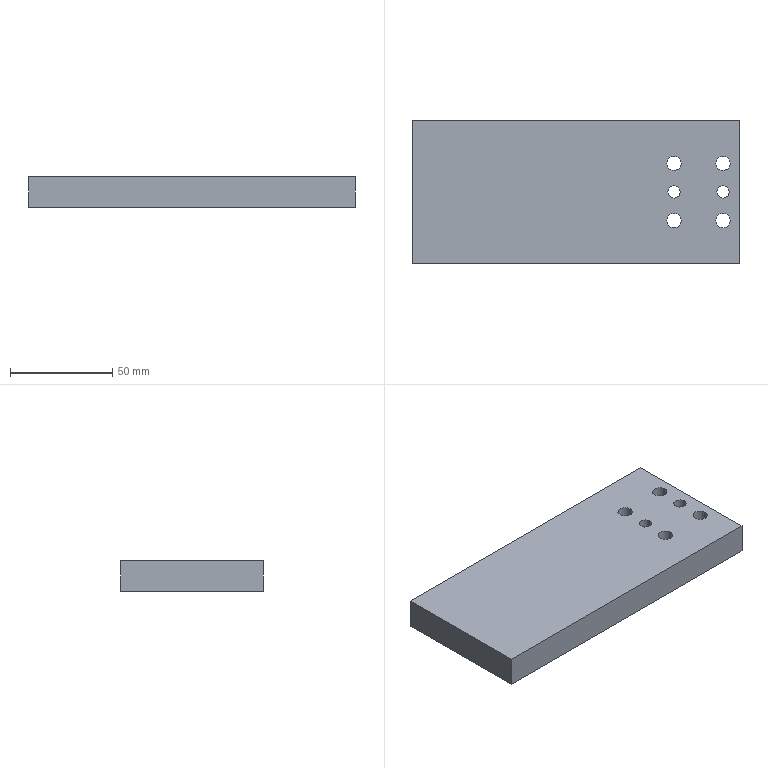Part | STEP file | Positioning_id1854_x_t | 1 solid | 18 faces | box 160 x 70 x 15 mm | volume 164843 mm3 | cylinder 12 | plane 6 | commonest cylinder face diameters 7 x8 6 x4